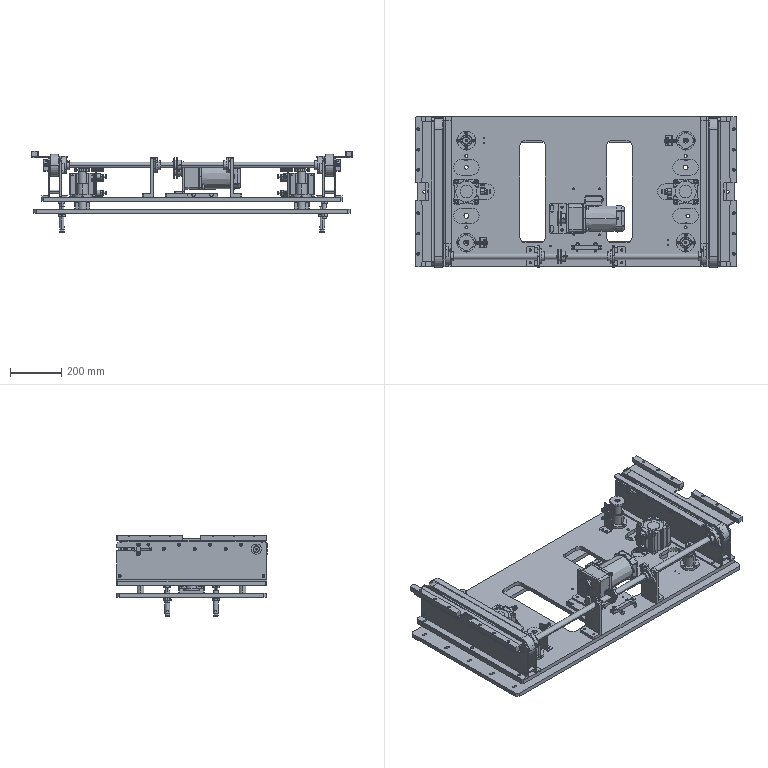Part | SolidWorks | 188 solids | 12377 faces | volume 27660270 mm3 | cylinder 4482 | plane 4336 | spline 2352 | cone 1137 | torus 54 | sphere 16 | commonest cylinder face diameters 12 x394 30.636 x288 0.2 x212 8.51 x184 11 x164 10 x160